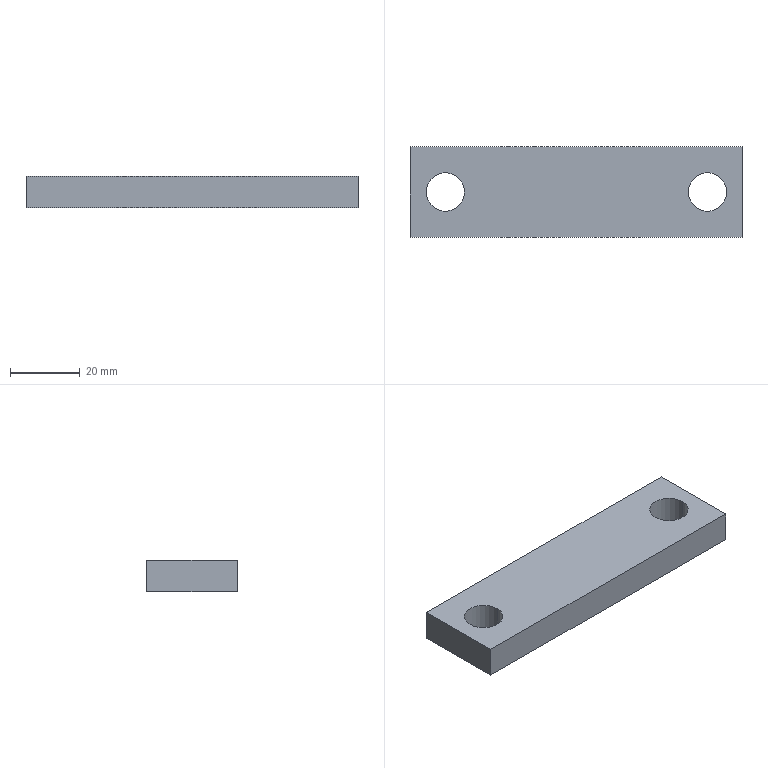Part | STEP file | 0244_205_Spacer | 1 solid | 10 faces | box 95 x 26 x 9 mm | volume 20519 mm3 | plane 6 | cylinder 4 | commonest cylinder face diameters 11 x4
STEP:
#1=CARTESIAN_POINT('',(0.,0.,0.));
#2=DIRECTION('',(0.,0.,1.));
#3=DIRECTION('',(1.,0.,0.));
#4=AXIS2_PLACEMENT_3D('',#1,#2,#3);
#5=CARTESIAN_POINT('',(-31.89,13.,0.));
#6=VERTEX_POINT('',#5);
#7=CARTESIAN_POINT('',(-31.89,13.,9.));
#8=VERTEX_POINT('',#7);
#9=CARTESIAN_POINT('',(-31.89,13.,9.));
#10=DIRECTION('',(0.,0.,1.));
#11=VECTOR('',#10,1.);
#12=LINE('',#9,#11);
#13=CARTESIAN_POINT('',(-37.39,13.,9.));
#14=DIRECTION('',(0.,0.,1.));
#15=DIRECTION('',(1.,0.,0.));
#16=AXIS2_PLACEMENT_3D('',#13,#14,#15);
#17=CYLINDRICAL_SURFACE('',#16,5.5);
#18=CARTESIAN_POINT('',(6.283,0.));
#19=DIRECTION('',(0.,1.));
#20=VECTOR('',#19,1.);
#21=LINE('',#18,#20);
#22=(GEOMETRIC_REPRESENTATION_CONTEXT(2)PARAMETRIC_REPRESENTATION_CONTEXT()REPRESENTATION_CONTEXT('',''));
#23=DEFINITIONAL_REPRESENTATION('',(#21),#22);
#24=PCURVE('',#17,#23);
#25=CARTESIAN_POINT('',(-37.39,13.,9.));
#26=DIRECTION('',(0.,0.,1.));
#27=DIRECTION('',(1.,0.,0.));
#28=AXIS2_PLACEMENT_3D('',#25,#26,#27);
#29=CYLINDRICAL_SURFACE('',#28,5.5);
#30=CARTESIAN_POINT('',(0.,0.));
#31=DIRECTION('',(0.,1.));
#32=VECTOR('',#31,1.);
#33=LINE('',#30,#32);
#34=(GEOMETRIC_REPRESENTATION_CONTEXT(2)PARAMETRIC_REPRESENTATION_CONTEXT()REPRESENTATION_CONTEXT('',''));
#35=DEFINITIONAL_REPRESENTATION('',(#33),#34);
#36=PCURVE('',#29,#35);
#37=SURFACE_CURVE('',#12,(#24,#36),.PCURVE_S1.);
#38=EDGE_CURVE('',#6,#8,#37,.T.);
#39=ORIENTED_EDGE('',*,*,#38,.T.);
#40=CARTESIAN_POINT('',(-42.89,13.,9.));
#41=VERTEX_POINT('',#40);
#42=CARTESIAN_POINT('',(-37.39,13.,9.));
#43=DIRECTION('',(0.,0.,1.));
#44=DIRECTION('',(1.,0.,0.));
#45=AXIS2_PLACEMENT_3D('',#42,#43,#44);
#46=CIRCLE('',#45,5.5);
#47=CARTESIAN_POINT('',(0.,0.));
#48=DIRECTION('',(1.,0.));
#49=VECTOR('',#48,1.);
#50=LINE('',#47,#49);
#51=(GEOMETRIC_REPRESENTATION_CONTEXT(2)PARAMETRIC_REPRESENTATION_CONTEXT()REPRESENTATION_CONTEXT('',''));
#52=DEFINITIONAL_REPRESENTATION('',(#50),#51);
#53=PCURVE('',#17,#52);
#54=CARTESIAN_POINT('',(-47.5,26.,9.));
#55=DIRECTION('',(0.,0.,-1.));
#56=DIRECTION('',(-1.,0.,0.));
#57=AXIS2_PLACEMENT_3D('',#54,#55,#56);
#58=PLANE('',#57);
#59=CARTESIAN_POINT('',(-15.61,-13.));
#60=CARTESIAN_POINT('',(-15.61,-3.474));
#61=CARTESIAN_POINT('',(-7.36,-8.237));
#62=CARTESIAN_POINT('',(0.8902,-13.));
#63=CARTESIAN_POINT('',(-7.36,-17.763));
#64=CARTESIAN_POINT('',(-15.61,-22.526));
#65=CARTESIAN_POINT('',(-15.61,-13.));
#66=(BOUNDED_CURVE()B_SPLINE_CURVE(2,(#59,#60,#61,#62,#63,#64,#65),.UNSPECIFIED.,.T.,.F.)B_SPLINE_CURVE_WITH_KNOTS((1,2,2,2,2,1),(-2.094,0.,2.094,4.189,6.283,8.378),.UNSPECIFIED.)CURVE()GEOMETRIC_REPRESENTATION_ITEM()RATIONAL_B_SPLINE_CURVE((1.,0.5,1.,0.5,1.,0.5,1.))REPRESENTATION_ITEM(''));
#67=(GEOMETRIC_REPRESENTATION_CONTEXT(2)PARAMETRIC_REPRESENTATION_CONTEXT()REPRESENTATION_CONTEXT('',''));
#68=DEFINITIONAL_REPRESENTATION('',(#66),#67);
#69=PCURVE('',#58,#68);
#70=SURFACE_CURVE('',#46,(#53,#69),.PCURVE_S1.);
#71=EDGE_CURVE('',#41,#8,#70,.T.);
#72=ORIENTED_EDGE('',*,*,#71,.F.);
#73=CARTESIAN_POINT('',(-42.89,13.,0.));
#74=VERTEX_POINT('',#73);
#75=CARTESIAN_POINT('',(-42.89,13.,9.));
#76=DIRECTION('',(0.,0.,1.));
#77=VECTOR('',#76,1.);
#78=LINE('',#75,#77);
#79=CARTESIAN_POINT('',(3.142,0.));
#80=DIRECTION('',(0.,1.));
#81=VECTOR('',#80,1.);
#82=LINE('',#79,#81);
#83=(GEOMETRIC_REPRESENTATION_CONTEXT(2)PARAMETRIC_REPRESENTATION_CONTEXT()REPRESENTATION_CONTEXT('',''));
#84=DEFINITIONAL_REPRESENTATION('',(#82),#83);
#85=PCURVE('',#17,#84);
#86=CARTESIAN_POINT('',(3.142,0.));
#87=DIRECTION('',(0.,1.));
#88=VECTOR('',#87,1.);
#89=LINE('',#86,#88);
#90=(GEOMETRIC_REPRESENTATION_CONTEXT(2)PARAMETRIC_REPRESENTATION_CONTEXT()REPRESENTATION_CONTEXT('',''));
#91=DEFINITIONAL_REPRESENTATION('',(#89),#90);
#92=PCURVE('',#29,#91);
#93=SURFACE_CURVE('',#78,(#85,#92),.PCURVE_S1.);
#94=EDGE_CURVE('',#74,#41,#93,.T.);
#95=ORIENTED_EDGE('',*,*,#94,.F.);
#96=CARTESIAN_POINT('',(-37.39,13.,0.));
#97=DIRECTION('',(0.,0.,1.));
#98=DIRECTION('',(1.,0.,0.));
#99=AXIS2_PLACEMENT_3D('',#96,#97,#98);
#100=CIRCLE('',#99,5.5);
#101=CARTESIAN_POINT('',(0.,-9.));
#102=DIRECTION('',(1.,0.));
#103=VECTOR('',#102,1.);
#104=LINE('',#101,#103);
#105=(GEOMETRIC_REPRESENTATION_CONTEXT(2)PARAMETRIC_REPRESENTATION_CONTEXT()REPRESENTATION_CONTEXT('',''));
#106=DEFINITIONAL_REPRESENTATION('',(#104),#105);
#107=PCURVE('',#17,#106);
#108=CARTESIAN_POINT('',(-47.5,26.,0.));
#109=DIRECTION('',(0.,0.,-1.));
#110=DIRECTION('',(-1.,0.,0.));
#111=AXIS2_PLACEMENT_3D('',#108,#109,#110);
#112=PLANE('',#111);
#113=CARTESIAN_POINT('',(-15.61,-13.));
#114=CARTESIAN_POINT('',(-15.61,-3.474));
#115=CARTESIAN_POINT('',(-7.36,-8.237));
#116=CARTESIAN_POINT('',(0.8902,-13.));
#117=CARTESIAN_POINT('',(-7.36,-17.763));
#118=CARTESIAN_POINT('',(-15.61,-22.526));
#119=CARTESIAN_POINT('',(-15.61,-13.));
#120=(BOUNDED_CURVE()B_SPLINE_CURVE(2,(#113,#114,#115,#116,#117,#118,#119),.UNSPECIFIED.,.T.,.F.)B_SPLINE_CURVE_WITH_KNOTS((1,2,2,2,2,1),(-2.094,0.,2.094,4.189,6.283,8.378),.UNSPECIFIED.)CURVE()GEOMETRIC_REPRESENTATION_ITEM()RATIONAL_B_SPLINE_CURVE((1.,0.5,1.,0.5,1.,0.5,1.))REPRESENTATION_ITEM(''));
#121=(GEOMETRIC_REPRESENTATION_CONTEXT(2)PARAMETRIC_REPRESENTATION_CONTEXT()REPRESENTATION_CONTEXT('',''));
#122=DEFINITIONAL_REPRESENTATION('',(#120),#121);
#123=PCURVE('',#112,#122);
#124=SURFACE_CURVE('',#100,(#107,#123),.PCURVE_S1.);
#125=EDGE_CURVE('',#74,#6,#124,.T.);
#126=ORIENTED_EDGE('',*,*,#125,.T.);
#127=EDGE_LOOP('',(#39,#72,#95,#126));
#128=FACE_BOUND('',#127,.F.);
#129=ADVANCED_FACE('',(#128),#17,.F.);
#130=CARTESIAN_POINT('',(43.11,13.,0.));
#131=VERTEX_POINT('',#130);
#132=CARTESIAN_POINT('',(43.11,13.,9.));
#133=VERTEX_POINT('',#132);
#134=CARTESIAN_POINT('',(43.11,13.,9.));
#135=DIRECTION('',(0.,0.,1.));
#136=VECTOR('',#135,1.);
#137=LINE('',#134,#136);
#138=CARTESIAN_POINT('',(37.61,13.,9.));
#139=DIRECTION('',(0.,0.,1.));
#140=DIRECTION('',(1.,0.,0.));
#141=AXIS2_PLACEMENT_3D('',#138,#139,#140);
#142=CYLINDRICAL_SURFACE('',#141,5.5);
#143=CARTESIAN_POINT('',(6.283,0.));
#144=DIRECTION('',(0.,1.));
#145=VECTOR('',#144,1.);
#146=LINE('',#143,#145);
#147=(GEOMETRIC_REPRESENTATION_CONTEXT(2)PARAMETRIC_REPRESENTATION_CONTEXT()REPRESENTATION_CONTEXT('',''));
#148=DEFINITIONAL_REPRESENTATION('',(#146),#147);
#149=PCURVE('',#142,#148);
#150=CARTESIAN_POINT('',(37.61,13.,9.));
#151=DIRECTION('',(0.,0.,1.));
#152=DIRECTION('',(1.,0.,0.));
#153=AXIS2_PLACEMENT_3D('',#150,#151,#152);
#154=CYLINDRICAL_SURFACE('',#153,5.5);
#155=CARTESIAN_POINT('',(0.,0.));
#156=DIRECTION('',(0.,1.));
#157=VECTOR('',#156,1.);
#158=LINE('',#155,#157);
#159=(GEOMETRIC_REPRESENTATION_CONTEXT(2)PARAMETRIC_REPRESENTATION_CONTEXT()REPRESENTATION_CONTEXT('',''));
#160=DEFINITIONAL_REPRESENTATION('',(#158),#159);
#161=PCURVE('',#154,#160);
#162=SURFACE_CURVE('',#137,(#149,#161),.PCURVE_S1.);
#163=EDGE_CURVE('',#131,#133,#162,.T.);
#164=ORIENTED_EDGE('',*,*,#163,.T.);
#165=CARTESIAN_POINT('',(32.11,13.,9.));
#166=VERTEX_POINT('',#165);
#167=CARTESIAN_POINT('',(37.61,13.,9.));
#168=DIRECTION('',(0.,0.,1.));
#169=DIRECTION('',(1.,0.,0.));
#170=AXIS2_PLACEMENT_3D('',#167,#168,#169);
#171=CIRCLE('',#170,5.5);
#172=CARTESIAN_POINT('',(0.,0.));
#173=DIRECTION('',(1.,0.));
#174=VECTOR('',#173,1.);
#175=LINE('',#172,#174);
#176=(GEOMETRIC_REPRESENTATION_CONTEXT(2)PARAMETRIC_REPRESENTATION_CONTEXT()REPRESENTATION_CONTEXT('',''));
#177=DEFINITIONAL_REPRESENTATION('',(#175),#176);
#178=PCURVE('',#142,#177);
#179=CARTESIAN_POINT('',(-90.61,-13.));
#180=CARTESIAN_POINT('',(-90.61,-3.474));
#181=CARTESIAN_POINT('',(-82.36,-8.237));
#182=CARTESIAN_POINT('',(-74.11,-13.));
#183=CARTESIAN_POINT('',(-82.36,-17.763));
#184=CARTESIAN_POINT('',(-90.61,-22.526));
#185=CARTESIAN_POINT('',(-90.61,-13.));
#186=(BOUNDED_CURVE()B_SPLINE_CURVE(2,(#179,#180,#181,#182,#183,#184,#185),.UNSPECIFIED.,.T.,.F.)B_SPLINE_CURVE_WITH_KNOTS((1,2,2,2,2,1),(-2.094,0.,2.094,4.189,6.283,8.378),.UNSPECIFIED.)CURVE()GEOMETRIC_REPRESENTATION_ITEM()RATIONAL_B_SPLINE_CURVE((1.,0.5,1.,0.5,1.,0.5,1.))REPRESENTATION_ITEM(''));
#187=(GEOMETRIC_REPRESENTATION_CONTEXT(2)PARAMETRIC_REPRESENTATION_CONTEXT()REPRESENTATION_CONTEXT('',''));
#188=DEFINITIONAL_REPRESENTATION('',(#186),#187);
#189=PCURVE('',#58,#188);
#190=SURFACE_CURVE('',#171,(#178,#189),.PCURVE_S1.);
#191=EDGE_CURVE('',#166,#133,#190,.T.);
#192=ORIENTED_EDGE('',*,*,#191,.F.);
#193=CARTESIAN_POINT('',(32.11,13.,0.));
#194=VERTEX_POINT('',#193);
#195=CARTESIAN_POINT('',(32.11,13.,9.));
#196=DIRECTION('',(0.,0.,1.));
#197=VECTOR('',#196,1.);
#198=LINE('',#195,#197);
#199=CARTESIAN_POINT('',(3.142,0.));
#200=DIRECTION('',(0.,1.));
#201=VECTOR('',#200,1.);
#202=LINE('',#199,#201);
#203=(GEOMETRIC_REPRESENTATION_CONTEXT(2)PARAMETRIC_REPRESENTATION_CONTEXT()REPRESENTATION_CONTEXT('',''));
#204=DEFINITIONAL_REPRESENTATION('',(#202),#203);
#205=PCURVE('',#142,#204);
#206=CARTESIAN_POINT('',(3.142,0.));
#207=DIRECTION('',(0.,1.));
#208=VECTOR('',#207,1.);
#209=LINE('',#206,#208);
#210=(GEOMETRIC_REPRESENTATION_CONTEXT(2)PARAMETRIC_REPRESENTATION_CONTEXT()REPRESENTATION_CONTEXT('',''));
#211=DEFINITIONAL_REPRESENTATION('',(#209),#210);
#212=PCURVE('',#154,#211);
#213=SURFACE_CURVE('',#198,(#205,#212),.PCURVE_S1.);
#214=EDGE_CURVE('',#194,#166,#213,.T.);
#215=ORIENTED_EDGE('',*,*,#214,.F.);
#216=CARTESIAN_POINT('',(37.61,13.,0.));
#217=DIRECTION('',(0.,0.,1.));
#218=DIRECTION('',(1.,0.,0.));
#219=AXIS2_PLACEMENT_3D('',#216,#217,#218);
#220=CIRCLE('',#219,5.5);
#221=CARTESIAN_POINT('',(0.,-9.));
#222=DIRECTION('',(1.,0.));
#223=VECTOR('',#222,1.);
#224=LINE('',#221,#223);
#225=(GEOMETRIC_REPRESENTATION_CONTEXT(2)PARAMETRIC_REPRESENTATION_CONTEXT()REPRESENTATION_CONTEXT('',''));
#226=DEFINITIONAL_REPRESENTATION('',(#224),#225);
#227=PCURVE('',#142,#226);
#228=CARTESIAN_POINT('',(-90.61,-13.));
#229=CARTESIAN_POINT('',(-90.61,-3.474));
#230=CARTESIAN_POINT('',(-82.36,-8.237));
#231=CARTESIAN_POINT('',(-74.11,-13.));
#232=CARTESIAN_POINT('',(-82.36,-17.763));
#233=CARTESIAN_POINT('',(-90.61,-22.526));
#234=CARTESIAN_POINT('',(-90.61,-13.));
#235=(BOUNDED_CURVE()B_SPLINE_CURVE(2,(#228,#229,#230,#231,#232,#233,#234),.UNSPECIFIED.,.T.,.F.)B_SPLINE_CURVE_WITH_KNOTS((1,2,2,2,2,1),(-2.094,0.,2.094,4.189,6.283,8.378),.UNSPECIFIED.)CURVE()GEOMETRIC_REPRESENTATION_ITEM()RATIONAL_B_SPLINE_CURVE((1.,0.5,1.,0.5,1.,0.5,1.))REPRESENTATION_ITEM(''));
#236=(GEOMETRIC_REPRESENTATION_CONTEXT(2)PARAMETRIC_REPRESENTATION_CONTEXT()REPRESENTATION_CONTEXT('',''));
#237=DEFINITIONAL_REPRESENTATION('',(#235),#236);
#238=PCURVE('',#112,#237);
#239=SURFACE_CURVE('',#220,(#227,#238),.PCURVE_S1.);
#240=EDGE_CURVE('',#194,#131,#239,.T.);
#241=ORIENTED_EDGE('',*,*,#240,.T.);
#242=EDGE_LOOP('',(#164,#192,#215,#241));
#243=FACE_BOUND('',#242,.F.);
#244=ADVANCED_FACE('',(#243),#142,.F.);
#245=CARTESIAN_POINT('',(-47.5,26.,0.));
#246=VERTEX_POINT('',#245);
#247=CARTESIAN_POINT('',(-47.5,0.,0.));
#248=VERTEX_POINT('',#247);
#249=CARTESIAN_POINT('',(-47.5,0.,0.));
#250=DIRECTION('',(0.,-1.,0.));
#251=VECTOR('',#250,1.);
#252=LINE('',#249,#251);
#253=CARTESIAN_POINT('',(-47.5,0.,9.));
#254=DIRECTION('',(1.,0.,0.));
#255=DIRECTION('',(0.,0.,-1.));
#256=AXIS2_PLACEMENT_3D('',#253,#254,#255);
#257=PLANE('',#256);
#258=CARTESIAN_POINT('',(9.,0.));
#259=DIRECTION('',(0.,-1.));
#260=VECTOR('',#259,1.);
#261=LINE('',#258,#260);
#262=(GEOMETRIC_REPRESENTATION_CONTEXT(2)PARAMETRIC_REPRESENTATION_CONTEXT()REPRESENTATION_CONTEXT('',''));
#263=DEFINITIONAL_REPRESENTATION('',(#261),#262);
#264=PCURVE('',#257,#263);
#265=CARTESIAN_POINT('',(0.,-26.));
#266=DIRECTION('',(0.,-1.));
#267=VECTOR('',#266,1.);
#268=LINE('',#265,#267);
#269=(GEOMETRIC_REPRESENTATION_CONTEXT(2)PARAMETRIC_REPRESENTATION_CONTEXT()REPRESENTATION_CONTEXT('',''));
#270=DEFINITIONAL_REPRESENTATION('',(#268),#269);
#271=PCURVE('',#112,#270);
#272=SURFACE_CURVE('',#252,(#264,#271),.PCURVE_S1.);
#273=EDGE_CURVE('',#246,#248,#272,.T.);
#274=ORIENTED_EDGE('',*,*,#273,.T.);
#275=CARTESIAN_POINT('',(-47.5,0.,9.));
#276=VERTEX_POINT('',#275);
#277=CARTESIAN_POINT('',(-47.5,0.,9.));
#278=DIRECTION('',(0.,0.,-1.));
#279=VECTOR('',#278,1.);
#280=LINE('',#277,#279);
#281=CARTESIAN_POINT('',(0.,0.));
#282=DIRECTION('',(1.,0.));
#283=VECTOR('',#282,1.);
#284=LINE('',#281,#283);
#285=(GEOMETRIC_REPRESENTATION_CONTEXT(2)PARAMETRIC_REPRESENTATION_CONTEXT()REPRESENTATION_CONTEXT('',''));
#286=DEFINITIONAL_REPRESENTATION('',(#284),#285);
#287=PCURVE('',#257,#286);
#288=CARTESIAN_POINT('',(-47.5,0.,9.));
#289=DIRECTION('',(0.,1.,0.));
#290=DIRECTION('',(0.,0.,1.));
#291=AXIS2_PLACEMENT_3D('',#288,#289,#290);
#292=PLANE('',#291);
#293=CARTESIAN_POINT('',(0.,0.));
#294=DIRECTION('',(-1.,0.));
#295=VECTOR('',#294,1.);
#296=LINE('',#293,#295);
#297=(GEOMETRIC_REPRESENTATION_CONTEXT(2)PARAMETRIC_REPRESENTATION_CONTEXT()REPRESENTATION_CONTEXT('',''));
#298=DEFINITIONAL_REPRESENTATION('',(#296),#297);
#299=PCURVE('',#292,#298);
#300=SURFACE_CURVE('',#280,(#287,#299),.PCURVE_S1.);
#301=EDGE_CURVE('',#276,#248,#300,.T.);
#302=ORIENTED_EDGE('',*,*,#301,.F.);
#303=CARTESIAN_POINT('',(-47.5,26.,9.));
#304=VERTEX_POINT('',#303);
#305=CARTESIAN_POINT('',(-47.5,0.,9.));
#306=DIRECTION('',(0.,-1.,0.));
#307=VECTOR('',#306,1.);
#308=LINE('',#305,#307);
#309=CARTESIAN_POINT('',(0.,0.));
#310=DIRECTION('',(0.,-1.));
#311=VECTOR('',#310,1.);
#312=LINE('',#309,#311);
#313=(GEOMETRIC_REPRESENTATION_CONTEXT(2)PARAMETRIC_REPRESENTATION_CONTEXT()REPRESENTATION_CONTEXT('',''));
#314=DEFINITIONAL_REPRESENTATION('',(#312),#313);
#315=PCURVE('',#257,#314);
#316=CARTESIAN_POINT('',(0.,-26.));
#317=DIRECTION('',(0.,-1.));
#318=VECTOR('',#317,1.);
#319=LINE('',#316,#318);
#320=(GEOMETRIC_REPRESENTATION_CONTEXT(2)PARAMETRIC_REPRESENTATION_CONTEXT()REPRESENTATION_CONTEXT('',''));
#321=DEFINITIONAL_REPRESENTATION('',(#319),#320);
#322=PCURVE('',#58,#321);
#323=SURFACE_CURVE('',#308,(#315,#322),.PCURVE_S1.);
#324=EDGE_CURVE('',#304,#276,#323,.T.);
#325=ORIENTED_EDGE('',*,*,#324,.F.);
#326=CARTESIAN_POINT('',(-47.5,26.,9.));
#327=DIRECTION('',(0.,0.,-1.));
#328=VECTOR('',#327,1.);
#329=LINE('',#326,#328);
#330=CARTESIAN_POINT('',(0.,26.));
#331=DIRECTION('',(1.,0.));
#332=VECTOR('',#331,1.);
#333=LINE('',#330,#332);
#334=(GEOMETRIC_REPRESENTATION_CONTEXT(2)PARAMETRIC_REPRESENTATION_CONTEXT()REPRESENTATION_CONTEXT('',''));
#335=DEFINITIONAL_REPRESENTATION('',(#333),#334);
#336=PCURVE('',#257,#335);
#337=CARTESIAN_POINT('',(-47.5,26.,9.));
#338=DIRECTION('',(0.,-1.,0.));
#339=DIRECTION('',(0.,0.,-1.));
#340=AXIS2_PLACEMENT_3D('',#337,#338,#339);
#341=PLANE('',#340);
#342=CARTESIAN_POINT('',(0.,0.));
#343=DIRECTION('',(1.,0.));
#344=VECTOR('',#343,1.);
#345=LINE('',#342,#344);
#346=(GEOMETRIC_REPRESENTATION_CONTEXT(2)PARAMETRIC_REPRESENTATION_CONTEXT()REPRESENTATION_CONTEXT('',''));
#347=DEFINITIONAL_REPRESENTATION('',(#345),#346);
#348=PCURVE('',#341,#347);
#349=SURFACE_CURVE('',#329,(#336,#348),.PCURVE_S1.);
#350=EDGE_CURVE('',#304,#246,#349,.T.);
#351=ORIENTED_EDGE('',*,*,#350,.T.);
#352=EDGE_LOOP('',(#274,#302,#325,#351));
#353=FACE_BOUND('',#352,.T.);
#354=ADVANCED_FACE('',(#353),#257,.F.);
#355=CARTESIAN_POINT('',(47.5,0.,0.));
#356=VERTEX_POINT('',#355);
#357=CARTESIAN_POINT('',(-47.5,0.,0.));
#358=DIRECTION('',(1.,0.,0.));
#359=VECTOR('',#358,1.);
#360=LINE('',#357,#359);
#361=CARTESIAN_POINT('',(-9.,0.));
#362=DIRECTION('',(0.,1.));
#363=VECTOR('',#362,1.);
#364=LINE('',#361,#363);
#365=(GEOMETRIC_REPRESENTATION_CONTEXT(2)PARAMETRIC_REPRESENTATION_CONTEXT()REPRESENTATION_CONTEXT('',''));
#366=DEFINITIONAL_REPRESENTATION('',(#364),#365);
#367=PCURVE('',#292,#366);
#368=CARTESIAN_POINT('',(0.,-26.));
#369=DIRECTION('',(-1.,0.));
#370=VECTOR('',#369,1.);
#371=LINE('',#368,#370);
#372=(GEOMETRIC_REPRESENTATION_CONTEXT(2)PARAMETRIC_REPRESENTATION_CONTEXT()REPRESENTATION_CONTEXT('',''));
#373=DEFINITIONAL_REPRESENTATION('',(#371),#372);
#374=PCURVE('',#112,#373);
#375=SURFACE_CURVE('',#360,(#367,#374),.PCURVE_S1.);
#376=EDGE_CURVE('',#248,#356,#375,.T.);
#377=ORIENTED_EDGE('',*,*,#376,.T.);
#378=CARTESIAN_POINT('',(47.5,0.,9.));
#379=VERTEX_POINT('',#378);
#380=CARTESIAN_POINT('',(47.5,0.,9.));
#381=DIRECTION('',(0.,0.,-1.));
#382=VECTOR('',#381,1.);
#383=LINE('',#380,#382);
#384=CARTESIAN_POINT('',(0.,95.));
#385=DIRECTION('',(-1.,0.));
#386=VECTOR('',#385,1.);
#387=LINE('',#384,#386);
#388=(GEOMETRIC_REPRESENTATION_CONTEXT(2)PARAMETRIC_REPRESENTATION_CONTEXT()REPRESENTATION_CONTEXT('',''));
#389=DEFINITIONAL_REPRESENTATION('',(#387),#388);
#390=PCURVE('',#292,#389);
#391=CARTESIAN_POINT('',(47.5,0.,9.));
#392=DIRECTION('',(-1.,0.,0.));
#393=DIRECTION('',(0.,0.,1.));
#394=AXIS2_PLACEMENT_3D('',#391,#392,#393);
#395=PLANE('',#394);
#396=CARTESIAN_POINT('',(0.,0.));
#397=DIRECTION('',(-1.,0.));
#398=VECTOR('',#397,1.);
#399=LINE('',#396,#398);
#400=(GEOMETRIC_REPRESENTATION_CONTEXT(2)PARAMETRIC_REPRESENTATION_CONTEXT()REPRESENTATION_CONTEXT('',''));
#401=DEFINITIONAL_REPRESENTATION('',(#399),#400);
#402=PCURVE('',#395,#401);
#403=SURFACE_CURVE('',#383,(#390,#402),.PCURVE_S1.);
#404=EDGE_CURVE('',#379,#356,#403,.T.);
#405=ORIENTED_EDGE('',*,*,#404,.F.);
#406=CARTESIAN_POINT('',(-47.5,0.,9.));
#407=DIRECTION('',(1.,0.,0.));
#408=VECTOR('',#407,1.);
#409=LINE('',#406,#408);
#410=CARTESIAN_POINT('',(0.,0.));
#411=DIRECTION('',(0.,1.));
#412=VECTOR('',#411,1.);
#413=LINE('',#410,#412);
#414=(GEOMETRIC_REPRESENTATION_CONTEXT(2)PARAMETRIC_REPRESENTATION_CONTEXT()REPRESENTATION_CONTEXT('',''));
#415=DEFINITIONAL_REPRESENTATION('',(#413),#414);
#416=PCURVE('',#292,#415);
#417=CARTESIAN_POINT('',(0.,-26.));
#418=DIRECTION('',(-1.,0.));
#419=VECTOR('',#418,1.);
#420=LINE('',#417,#419);
#421=(GEOMETRIC_REPRESENTATION_CONTEXT(2)PARAMETRIC_REPRESENTATION_CONTEXT()REPRESENTATION_CONTEXT('',''));
#422=DEFINITIONAL_REPRESENTATION('',(#420),#421);
#423=PCURVE('',#58,#422);
#424=SURFACE_CURVE('',#409,(#416,#423),.PCURVE_S1.);
#425=EDGE_CURVE('',#276,#379,#424,.T.);
#426=ORIENTED_EDGE('',*,*,#425,.F.);
#427=ORIENTED_EDGE('',*,*,#301,.T.);
#428=EDGE_LOOP('',(#377,#405,#426,#427));
#429=FACE_BOUND('',#428,.T.);
#430=ADVANCED_FACE('',(#429),#292,.F.);
#431=CARTESIAN_POINT('',(47.5,26.,0.));
#432=VERTEX_POINT('',#431);
#433=CARTESIAN_POINT('',(47.5,0.,0.));
#434=DIRECTION('',(0.,1.,0.));
#435=VECTOR('',#434,1.);
#436=LINE('',#433,#435);
#437=CARTESIAN_POINT('',(-9.,0.));
#438=DIRECTION('',(0.,1.));
#439=VECTOR('',#438,1.);
#440=LINE('',#437,#439);
#441=(GEOMETRIC_REPRESENTATION_CONTEXT(2)PARAMETRIC_REPRESENTATION_CONTEXT()REPRESENTATION_CONTEXT('',''));
#442=DEFINITIONAL_REPRESENTATION('',(#440),#441);
#443=PCURVE('',#395,#442);
#444=CARTESIAN_POINT('',(-95.,-26.));
#445=DIRECTION('',(0.,1.));
#446=VECTOR('',#445,1.);
#447=LINE('',#444,#446);
#448=(GEOMETRIC_REPRESENTATION_CONTEXT(2)PARAMETRIC_REPRESENTATION_CONTEXT()REPRESENTATION_CONTEXT('',''));
#449=DEFINITIONAL_REPRESENTATION('',(#447),#448);
#450=PCURVE('',#112,#449);
#451=SURFACE_CURVE('',#436,(#443,#450),.PCURVE_S1.);
#452=EDGE_CURVE('',#356,#432,#451,.T.);
#453=ORIENTED_EDGE('',*,*,#452,.T.);
#454=CARTESIAN_POINT('',(47.5,26.,9.));
#455=VERTEX_POINT('',#454);
#456=CARTESIAN_POINT('',(47.5,26.,9.));
#457=DIRECTION('',(0.,0.,-1.));
#458=VECTOR('',#457,1.);
#459=LINE('',#456,#458);
#460=CARTESIAN_POINT('',(0.,26.));
#461=DIRECTION('',(-1.,0.));
#462=VECTOR('',#461,1.);
#463=LINE('',#460,#462);
#464=(GEOMETRIC_REPRESENTATION_CONTEXT(2)PARAMETRIC_REPRESENTATION_CONTEXT()REPRESENTATION_CONTEXT('',''));
#465=DEFINITIONAL_REPRESENTATION('',(#463),#464);
#466=PCURVE('',#395,#465);
#467=CARTESIAN_POINT('',(0.,95.));
#468=DIRECTION('',(1.,0.));
#469=VECTOR('',#468,1.);
#470=LINE('',#467,#469);
#471=(GEOMETRIC_REPRESENTATION_CONTEXT(2)PARAMETRIC_REPRESENTATION_CONTEXT()REPRESENTATION_CONTEXT('',''));
#472=DEFINITIONAL_REPRESENTATION('',(#470),#471);
#473=PCURVE('',#341,#472);
#474=SURFACE_CURVE('',#459,(#466,#473),.PCURVE_S1.);
#475=EDGE_CURVE('',#455,#432,#474,.T.);
#476=ORIENTED_EDGE('',*,*,#475,.F.);
#477=CARTESIAN_POINT('',(47.5,0.,9.));
#478=DIRECTION('',(0.,1.,0.));
#479=VECTOR('',#478,1.);
#480=LINE('',#477,#479);
#481=CARTESIAN_POINT('',(0.,0.));
#482=DIRECTION('',(0.,1.));
#483=VECTOR('',#482,1.);
#484=LINE('',#481,#483);
#485=(GEOMETRIC_REPRESENTATION_CONTEXT(2)PARAMETRIC_REPRESENTATION_CONTEXT()REPRESENTATION_CONTEXT('',''));
#486=DEFINITIONAL_REPRESENTATION('',(#484),#485);
#487=PCURVE('',#395,#486);
#488=CARTESIAN_POINT('',(-95.,-26.));
#489=DIRECTION('',(0.,1.));
#490=VECTOR('',#489,1.);
#491=LINE('',#488,#490);
#492=(GEOMETRIC_REPRESENTATION_CONTEXT(2)PARAMETRIC_REPRESENTATION_CONTEXT()REPRESENTATION_CONTEXT('',''));
#493=DEFINITIONAL_REPRESENTATION('',(#491),#492);
#494=PCURVE('',#58,#493);
#495=SURFACE_CURVE('',#480,(#487,#494),.PCURVE_S1.);
#496=EDGE_CURVE('',#379,#455,#495,.T.);
#497=ORIENTED_EDGE('',*,*,#496,.F.);
#498=ORIENTED_EDGE('',*,*,#404,.T.);
#499=EDGE_LOOP('',(#453,#476,#497,#498));
#500=FACE_BOUND('',#499,.T.);
#501=ADVANCED_FACE('',(#500),#395,.F.);
#502=CARTESIAN_POINT('',(-47.5,26.,0.));
#503=DIRECTION('',(-1.,0.,0.));
#504=VECTOR('',#503,1.);
#505=LINE('',#502,#504);
#506=CARTESIAN_POINT('',(9.,0.));
#507=DIRECTION('',(0.,-1.));
#508=VECTOR('',#507,1.);
#509=LINE('',#506,#508);
#510=(GEOMETRIC_REPRESENTATION_CONTEXT(2)PARAMETRIC_REPRESENTATION_CONTEXT()REPRESENTATION_CONTEXT('',''));
#511=DEFINITIONAL_REPRESENTATION('',(#509),#510);
#512=PCURVE('',#341,#511);
#513=CARTESIAN_POINT('',(0.,0.));
#514=DIRECTION('',(1.,0.));
#515=VECTOR('',#514,1.);
#516=LINE('',#513,#515);
#517=(GEOMETRIC_REPRESENTATION_CONTEXT(2)PARAMETRIC_REPRESENTATION_CONTEXT()REPRESENTATION_CONTEXT('',''));
#518=DEFINITIONAL_REPRESENTATION('',(#516),#517);
#519=PCURVE('',#112,#518);
#520=SURFACE_CURVE('',#505,(#512,#519),.PCURVE_S1.);
#521=EDGE_CURVE('',#432,#246,#520,.T.);
#522=ORIENTED_EDGE('',*,*,#521,.T.);
#523=ORIENTED_EDGE('',*,*,#350,.F.);
#524=CARTESIAN_POINT('',(-47.5,26.,9.));
#525=DIRECTION('',(-1.,0.,0.));
#526=VECTOR('',#525,1.);
#527=LINE('',#524,#526);
#528=CARTESIAN_POINT('',(0.,0.));
#529=DIRECTION('',(0.,-1.));
#530=VECTOR('',#529,1.);
#531=LINE('',#528,#530);
#532=(GEOMETRIC_REPRESENTATION_CONTEXT(2)PARAMETRIC_REPRESENTATION_CONTEXT()REPRESENTATION_CONTEXT('',''));
#533=DEFINITIONAL_REPRESENTATION('',(#531),#532);
#534=PCURVE('',#341,#533);
#535=CARTESIAN_POINT('',(0.,0.));
#536=DIRECTION('',(1.,0.));
#537=VECTOR('',#536,1.);
#538=LINE('',#535,#537);
#539=(GEOMETRIC_REPRESENTATION_CONTEXT(2)PARAMETRIC_REPRESENTATION_CONTEXT()REPRESENTATION_CONTEXT('',''));
#540=DEFINITIONAL_REPRESENTATION('',(#538),#539);
#541=PCURVE('',#58,#540);
#542=SURFACE_CURVE('',#527,(#534,#541),.PCURVE_S1.);
#543=EDGE_CURVE('',#455,#304,#542,.T.);
#544=ORIENTED_EDGE('',*,*,#543,.F.);
#545=ORIENTED_EDGE('',*,*,#475,.T.);
#546=EDGE_LOOP('',(#522,#523,#544,#545));
#547=FACE_BOUND('',#546,.T.);
#548=ADVANCED_FACE('',(#547),#341,.F.);
#549=CARTESIAN_POINT('',(-37.39,13.,9.));
#550=DIRECTION('',(0.,0.,1.));
#551=DIRECTION('',(1.,0.,0.));
#552=AXIS2_PLACEMENT_3D('',#549,#550,#551);
#553=CIRCLE('',#552,5.5);
#554=CARTESIAN_POINT('',(-15.61,-13.));
#555=CARTESIAN_POINT('',(-15.61,-3.474));
#556=CARTESIAN_POINT('',(-7.36,-8.237));
#557=CARTESIAN_POINT('',(0.8902,-13.));
#558=CARTESIAN_POINT('',(-7.36,-17.763));
#559=CARTESIAN_POINT('',(-15.61,-22.526));
#560=CARTESIAN_POINT('',(-15.61,-13.));
#561=(BOUNDED_CURVE()B_SPLINE_CURVE(2,(#554,#555,#556,#557,#558,#559,#560),.UNSPECIFIED.,.T.,.F.)B_SPLINE_CURVE_WITH_KNOTS((1,2,2,2,2,1),(-2.094,0.,2.094,4.189,6.283,8.378),.UNSPECIFIED.)CURVE()GEOMETRIC_REPRESENTATION_ITEM()RATIONAL_B_SPLINE_CURVE((1.,0.5,1.,0.5,1.,0.5,1.))REPRESENTATION_ITEM(''));
#562=(GEOMETRIC_REPRESENTATION_CONTEXT(2)PARAMETRIC_REPRESENTATION_CONTEXT()REPRESENTATION_CONTEXT('',''));
#563=DEFINITIONAL_REPRESENTATION('',(#561),#562);
#564=PCURVE('',#58,#563);
#565=CARTESIAN_POINT('',(0.,0.));
#566=DIRECTION('',(1.,0.));
#567=VECTOR('',#566,1.);
#568=LINE('',#565,#567);
#569=(GEOMETRIC_REPRESENTATION_CONTEXT(2)PARAMETRIC_REPRESENTATION_CONTEXT()REPRESENTATION_CONTEXT('',''));
#570=DEFINITIONAL_REPRESENTATION('',(#568),#569);
#571=PCURVE('',#29,#570);
#572=SURFACE_CURVE('',#553,(#564,#571),.PCURVE_S1.);
#573=EDGE_CURVE('',#8,#41,#572,.T.);
#574=ORIENTED_EDGE('',*,*,#573,.F.);
#575=ORIENTED_EDGE('',*,*,#71,.F.);
#576=EDGE_LOOP('',(#574,#575));
#577=FACE_BOUND('',#576,.T.);
#578=CARTESIAN_POINT('',(37.61,13.,9.));
#579=DIRECTION('',(0.,0.,1.));
#580=DIRECTION('',(1.,0.,0.));
#581=AXIS2_PLACEMENT_3D('',#578,#579,#580);
#582=CIRCLE('',#581,5.5);
#583=CARTESIAN_POINT('',(-90.61,-13.));
#584=CARTESIAN_POINT('',(-90.61,-3.474));
#585=CARTESIAN_POINT('',(-82.36,-8.237));
#586=CARTESIAN_POINT('',(-74.11,-13.));
#587=CARTESIAN_POINT('',(-82.36,-17.763));
#588=CARTESIAN_POINT('',(-90.61,-22.526));
#589=CARTESIAN_POINT('',(-90.61,-13.));
#590=(BOUNDED_CURVE()B_SPLINE_CURVE(2,(#583,#584,#585,#586,#587,#588,#589),.UNSPECIFIED.,.T.,.F.)B_SPLINE_CURVE_WITH_KNOTS((1,2,2,2,2,1),(-2.094,0.,2.094,4.189,6.283,8.378),.UNSPECIFIED.)CURVE()GEOMETRIC_REPRESENTATION_ITEM()RATIONAL_B_SPLINE_CURVE((1.,0.5,1.,0.5,1.,0.5,1.))REPRESENTATION_ITEM(''));
#591=(GEOMETRIC_REPRESENTATION_CONTEXT(2)PARAMETRIC_REPRESENTATION_CONTEXT()REPRESENTATION_CONTEXT('',''));
#592=DEFINITIONAL_REPRESENTATION('',(#590),#591);
#593=PCURVE('',#58,#592);
#594=CARTESIAN_POINT('',(0.,0.));
#595=DIRECTION('',(1.,0.));
#596=VECTOR('',#595,1.);
#597=LINE('',#594,#596);
#598=(GEOMETRIC_REPRESENTATION_CONTEXT(2)PARAMETRIC_REPRESENTATION_CONTEXT()REPRESENTATION_CONTEXT('',''));
#599=DEFINITIONAL_REPRESENTATION('',(#597),#598);
#600=PCURVE('',#154,#599);
#601=SURFACE_CURVE('',#582,(#593,#600),.PCURVE_S1.);
#602=EDGE_CURVE('',#133,#166,#601,.T.);
#603=ORIENTED_EDGE('',*,*,#602,.F.);
#604=ORIENTED_EDGE('',*,*,#191,.F.);
#605=EDGE_LOOP('',(#603,#604));
#606=FACE_BOUND('',#605,.T.);
#607=ORIENTED_EDGE('',*,*,#324,.T.);
#608=ORIENTED_EDGE('',*,*,#425,.T.);
#609=ORIENTED_EDGE('',*,*,#496,.T.);
#610=ORIENTED_EDGE('',*,*,#543,.T.);
#611=EDGE_LOOP('',(#607,#608,#609,#610));
#612=FACE_BOUND('',#611,.T.);
#613=ADVANCED_FACE('',(#577,#606,#612),#58,.F.);
#614=CARTESIAN_POINT('',(-37.39,13.,0.));
#615=DIRECTION('',(0.,0.,1.));
#616=DIRECTION('',(1.,0.,0.));
#617=AXIS2_PLACEMENT_3D('',#614,#615,#616);
#618=CIRCLE('',#617,5.5);
#619=CARTESIAN_POINT('',(-15.61,-13.));
#620=CARTESIAN_POINT('',(-15.61,-3.474));
#621=CARTESIAN_POINT('',(-7.36,-8.237));
#622=CARTESIAN_POINT('',(0.8902,-13.));
#623=CARTESIAN_POINT('',(-7.36,-17.763));
#624=CARTESIAN_POINT('',(-15.61,-22.526));
#625=CARTESIAN_POINT('',(-15.61,-13.));
#626=(BOUNDED_CURVE()B_SPLINE_CURVE(2,(#619,#620,#621,#622,#623,#624,#625),.UNSPECIFIED.,.T.,.F.)B_SPLINE_CURVE_WITH_KNOTS((1,2,2,2,2,1),(-2.094,0.,2.094,4.189,6.283,8.378),.UNSPECIFIED.)CURVE()GEOMETRIC_REPRESENTATION_ITEM()RATIONAL_B_SPLINE_CURVE((1.,0.5,1.,0.5,1.,0.5,1.))REPRESENTATION_ITEM(''));
#627=(GEOMETRIC_REPRESENTATION_CONTEXT(2)PARAMETRIC_REPRESENTATION_CONTEXT()REPRESENTATION_CONTEXT('',''));
#628=DEFINITIONAL_REPRESENTATION('',(#626),#627);
#629=PCURVE('',#112,#628);
#630=CARTESIAN_POINT('',(0.,-9.));
#631=DIRECTION('',(1.,0.));
#632=VECTOR('',#631,1.);
#633=LINE('',#630,#632);
#634=(GEOMETRIC_REPRESENTATION_CONTEXT(2)PARAMETRIC_REPRESENTATION_CONTEXT()REPRESENTATION_CONTEXT('',''));
#635=DEFINITIONAL_REPRESENTATION('',(#633),#634);
#636=PCURVE('',#29,#635);
#637=SURFACE_CURVE('',#618,(#629,#636),.PCURVE_S1.);
#638=EDGE_CURVE('',#6,#74,#637,.T.);
#639=ORIENTED_EDGE('',*,*,#638,.T.);
#640=ORIENTED_EDGE('',*,*,#125,.T.);
#641=EDGE_LOOP('',(#639,#640));
#642=FACE_BOUND('',#641,.T.);
#643=CARTESIAN_POINT('',(37.61,13.,0.));
#644=DIRECTION('',(0.,0.,1.));
#645=DIRECTION('',(1.,0.,0.));
#646=AXIS2_PLACEMENT_3D('',#643,#644,#645);
#647=CIRCLE('',#646,5.5);
#648=CARTESIAN_POINT('',(-90.61,-13.));
#649=CARTESIAN_POINT('',(-90.61,-3.474));
#650=CARTESIAN_POINT('',(-82.36,-8.237));
#651=CARTESIAN_POINT('',(-74.11,-13.));
#652=CARTESIAN_POINT('',(-82.36,-17.763));
#653=CARTESIAN_POINT('',(-90.61,-22.526));
#654=CARTESIAN_POINT('',(-90.61,-13.));
#655=(BOUNDED_CURVE()B_SPLINE_CURVE(2,(#648,#649,#650,#651,#652,#653,#654),.UNSPECIFIED.,.T.,.F.)B_SPLINE_CURVE_WITH_KNOTS((1,2,2,2,2,1),(-2.094,0.,2.094,4.189,6.283,8.378),.UNSPECIFIED.)CURVE()GEOMETRIC_REPRESENTATION_ITEM()RATIONAL_B_SPLINE_CURVE((1.,0.5,1.,0.5,1.,0.5,1.))REPRESENTATION_ITEM(''));
#656=(GEOMETRIC_REPRESENTATION_CONTEXT(2)PARAMETRIC_REPRESENTATION_CONTEXT()REPRESENTATION_CONTEXT('',''));
#657=DEFINITIONAL_REPRESENTATION('',(#655),#656);
#658=PCURVE('',#112,#657);
#659=CARTESIAN_POINT('',(0.,-9.));
#660=DIRECTION('',(1.,0.));
#661=VECTOR('',#660,1.);
#662=LINE('',#659,#661);
#663=(GEOMETRIC_REPRESENTATION_CONTEXT(2)PARAMETRIC_REPRESENTATION_CONTEXT()REPRESENTATION_CONTEXT('',''));
#664=DEFINITIONAL_REPRESENTATION('',(#662),#663);
#665=PCURVE('',#154,#664);
#666=SURFACE_CURVE('',#647,(#658,#665),.PCURVE_S1.);
#667=EDGE_CURVE('',#131,#194,#666,.T.);
#668=ORIENTED_EDGE('',*,*,#667,.T.);
#669=ORIENTED_EDGE('',*,*,#240,.T.);
#670=EDGE_LOOP('',(#668,#669));
#671=FACE_BOUND('',#670,.T.);
#672=ORIENTED_EDGE('',*,*,#273,.F.);
#673=ORIENTED_EDGE('',*,*,#521,.F.);
#674=ORIENTED_EDGE('',*,*,#452,.F.);
#675=ORIENTED_EDGE('',*,*,#376,.F.);
#676=EDGE_LOOP('',(#672,#673,#674,#675));
#677=FACE_BOUND('',#676,.T.);
#678=ADVANCED_FACE('',(#642,#671,#677),#112,.T.);
#679=ORIENTED_EDGE('',*,*,#602,.F.);
#680=ORIENTED_EDGE('',*,*,#163,.F.);
#681=ORIENTED_EDGE('',*,*,#667,.T.);
#682=ORIENTED_EDGE('',*,*,#214,.T.);
#683=EDGE_LOOP('',(#679,#680,#681,#682));
#684=FACE_BOUND('',#683,.F.);
#685=ADVANCED_FACE('',(#684),#154,.F.);
#686=ORIENTED_EDGE('',*,*,#573,.F.);
#687=ORIENTED_EDGE('',*,*,#38,.F.);
#688=ORIENTED_EDGE('',*,*,#638,.T.);
#689=ORIENTED_EDGE('',*,*,#94,.T.);
#690=EDGE_LOOP('',(#686,#687,#688,#689));
#691=FACE_BOUND('',#690,.F.);
#692=ADVANCED_FACE('',(#691),#29,.F.);
#693=CLOSED_SHELL('',(#129,#244,#354,#430,#501,#548,#613,#678,#685,#692));
#694=MANIFOLD_SOLID_BREP('',#693);
#695=(LENGTH_UNIT()NAMED_UNIT(*)SI_UNIT(.MILLI.,.METRE.));
#696=UNCERTAINTY_MEASURE_WITH_UNIT(LENGTH_MEASURE(0.0000001),#695,'','');
#697=(NAMED_UNIT(*)PLANE_ANGLE_UNIT()SI_UNIT($,.RADIAN.));
#698=(NAMED_UNIT(*)SI_UNIT($,.STERADIAN.)SOLID_ANGLE_UNIT());
#699=(GEOMETRIC_REPRESENTATION_CONTEXT(3)GLOBAL_UNCERTAINTY_ASSIGNED_CONTEXT((#696))GLOBAL_UNIT_ASSIGNED_CONTEXT((#695,#697,#698))REPRESENTATION_CONTEXT('',''));
#700=ADVANCED_BREP_SHAPE_REPRESENTATION('',(#4,#694),#699);